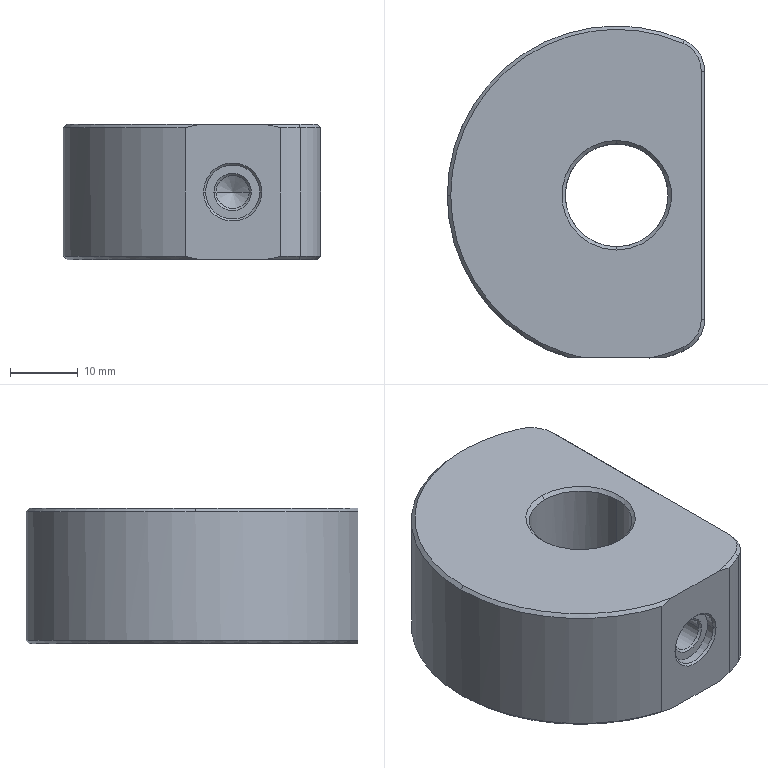Part | STEP file | Pressure roller | 1 solid | 36 faces | box 38 x 49 x 20 mm | volume 27809 mm3 | cone 19 | cylinder 10 | plane 7 | commonest cylinder face diameters 4.917 x2 8 x2 10 x2 15.2 x2 50 x2